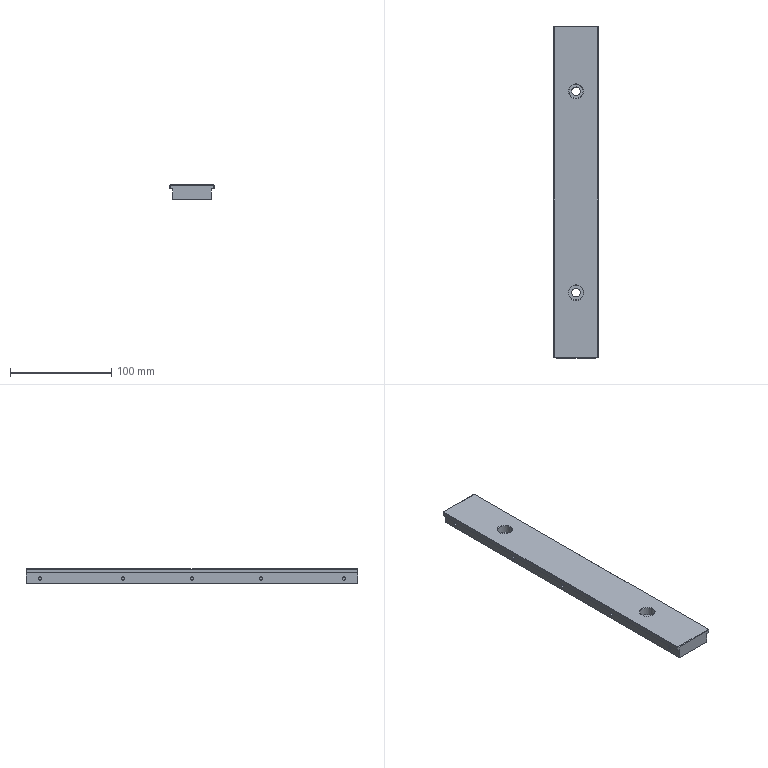CAM job | NX | 3-axis milling, drilling | part box 44 x 328 x 14 mm | stock box 45 x 333 x 20 mm
Tools:
number,name,description,diameter,corner_radius,flute_length,length,flutes
6,D6,平底铣刀-粗,6.0,0.0,25.0,75.0,2
9,D10,平底铣刀-粗,10.0,0.0,35.0,75.0,2
7,D6-J,平底铣刀-精,6.0,0.0,25.0,75.0,2
10,D10-J,平底铣刀-精,10.0,0.0,35.0,75.0,2
1,D80R0.8飞刀,圆鼻刀-粗,80.0,0.8,50.0,75.0,2
1,D80R0.8飞刀-J,圆鼻刀-精,80.0,0.8,50.0,75.0,2
2,D6倒角刀,倒角刀,6.0,0.0,3.0,25.0,2
17,ZT8.5,钻头,8.5,0.0,35.0,50.0,2
Operations:
program,operation,operation_type,tool,method,geometry_group,spindle_rpm,surface_speed,feed_per_tooth,feed_cut,feed_plunge,cut_length_mm,path_length_mm,cut_time_min,machine_time_min
B,底壁铣飞面一刀开粗_COPY,VolumeBased25DMillingOperation,D80R0.8飞刀,分层开粗-切深K-步距G,W-B,2800.0,703.696,0.5357,3000.0,100.0,4798.134,9377.511,1.599,2.057
B,底壁铣飞面一刀精光_COPY,VolumeBased25DMillingOperation,D80R0.8飞刀-J,侧刃精光-切深K-步距G,W-B,4000.0,1005.28,0.125,1000.0,100.0,435.998,471.998,0.436,0.4396
B,铣沉头_1,CylinderMilling,D6,METHOD,W-B,8000.0,150.796,0.1562,2500.0,100.0,496.414,544.114,0.1986,0.2033
B,铣沉头_2,CylinderMilling,D6,METHOD,W-B,8000.0,150.796,0.1562,2500.0,100.0,527.982,575.682,0.2112,0.216
B,铣孔_1,CylinderMilling,D6-J,METHOD,W-B,8000.0,150.796,0.05,800.0,100.0,68.139,125.139,0.0852,0.0909
B,铣孔_2,CylinderMilling,D6-J,METHOD,W-B,8000.0,150.796,0.05,800.0,100.0,72.279,129.279,0.0903,0.096
B,底壁铣倒角_COPY,VolumeBased25DMillingOperation,D6倒角刀,爬面_倒角-切深0-步距G,W-B,6500.0,122.519,0.1154,1500.0,100.0,849.689,1297.841,0.5665,0.6113
A,顶面,FaceMilling,D80R0.8飞刀,侧刃精光-切深K-步距G,W-A,5000.0,1256.637,0.1,1000.0,100.0,422.0,458.0,0.422,0.4256
A,外形粗_2,VolumeBased25DMillingOperation,D10,METHOD,W-A,8000.0,251.327,0.3125,5000.0,80.0,15498.961,15551.461,3.1,3.105
A,等高往复层切开粗-中_COPY,ZLevelMilling,D10,分层开粗-切深K-步距G,W-A,8000.0,251.327,0.375,6000.0,100.0,11053.939,11520.354,1.842,1.889
A,打点-深0.8,Operation,D6倒角刀,NONE,W-A,8000.0,150.796,0.0312,500.0,90.0,3.6,247.202,0.0072,0.0316
A,通孔-8-10,Operation,ZT8.5,NONE,W-A,1800.0,48.066,0.0833,300.0,90.0,38.0,316.002,0.1267,0.1545
A,底壁铣螺旋开粗-中_COPY,VolumeBased25DMillingOperation,D6,分层开粗-切深K-步距G,W-A,8000.0,150.796,0.0938,1500.0,100.0,596.213,863.2,0.3975,0.4242
A,仅选体,SurfaceContour,D6倒角刀,METHOD,W-A,8000.0,150.796,0.1875,3000.0,100.0,1467.319,1792.668,0.4891,0.5216
A,铣倒角_1,PlanarMilling,D6倒角刀,METHOD,W-A,8000.0,150.796,0.05,800.0,100.0,67.46,348.244,0.0843,0.1124
A,底侧精_3,VolumeBased25DMillingOperation,D6-J,METHOD,W-A,6000.0,113.0,0.2083,1200.0,100.0,1350.966,2283.866,1.126,1.219
A,底侧精_4,VolumeBased25DMillingOperation,D6-J,METHOD,W-A,6000.0,113.0,0.2083,1200.0,100.0,90.253,374.553,0.0752,0.1036
A,外形半精_2,VolumeBased25DMillingOperation,D10-J,METHOD,W-A,8000.0,251.327,0.0625,1000.0,100.0,779.202,846.202,0.7792,0.7859